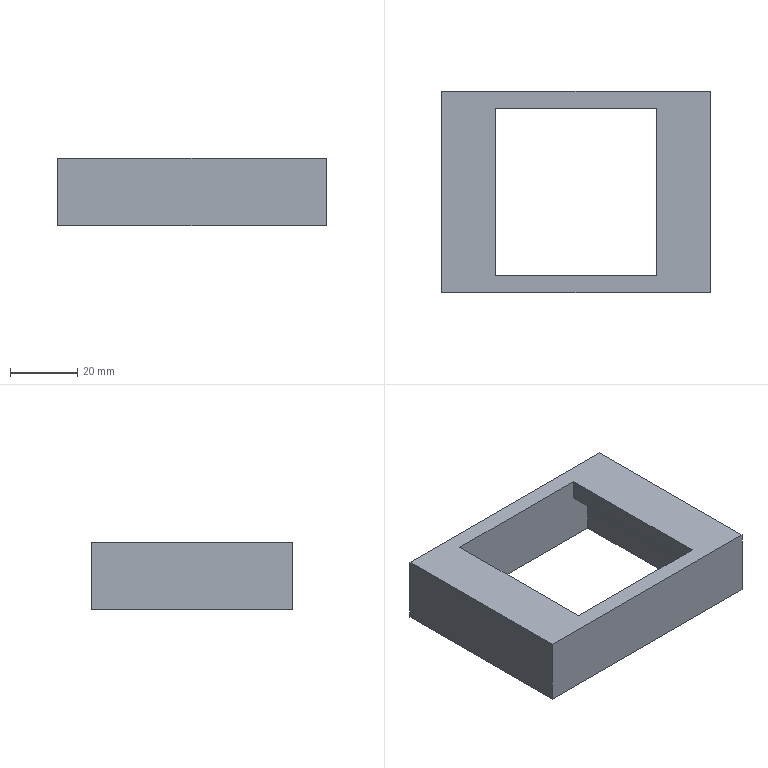Part | SolidWorks | features ICE 2, Extrusion 1 | 1 solid | 14 faces | box 80 x 60 x 20 mm | volume 39600 mm3 | plane 14
STEP:
#1=CARTESIAN_POINT('',(-24.,25.,14.));
#2=VERTEX_POINT('',#1);
#3=CARTESIAN_POINT('',(-24.,-25.,14.));
#4=VERTEX_POINT('',#3);
#5=CARTESIAN_POINT('',(-24.,-25.,14.));
#6=DIRECTION('',(0.,-1.,0.));
#7=VECTOR('',#6,1000.);
#8=LINE('',#5,#7);
#9=EDGE_CURVE('',#2,#4,#8,.T.);
#10=ORIENTED_EDGE('',*,*,#9,.F.);
#11=CARTESIAN_POINT('',(-24.,25.,20.));
#12=VERTEX_POINT('',#11);
#13=CARTESIAN_POINT('',(-24.,25.,-0.001));
#14=DIRECTION('',(0.,0.,1.));
#15=VECTOR('',#14,1000.);
#16=LINE('',#13,#15);
#17=EDGE_CURVE('',#2,#12,#16,.T.);
#18=ORIENTED_EDGE('',*,*,#17,.T.);
#19=CARTESIAN_POINT('',(-24.,-25.,20.));
#20=VERTEX_POINT('',#19);
#21=CARTESIAN_POINT('',(-24.,-25.,20.));
#22=DIRECTION('',(0.,-1.,0.));
#23=VECTOR('',#22,1000.);
#24=LINE('',#21,#23);
#25=EDGE_CURVE('',#12,#20,#24,.T.);
#26=ORIENTED_EDGE('',*,*,#25,.T.);
#27=CARTESIAN_POINT('',(-24.,-25.,-0.001));
#28=DIRECTION('',(0.,0.,1.));
#29=VECTOR('',#28,1000.);
#30=LINE('',#27,#29);
#31=EDGE_CURVE('',#4,#20,#30,.T.);
#32=ORIENTED_EDGE('',*,*,#31,.F.);
#33=EDGE_LOOP('',(#10,#18,#26,#32));
#34=FACE_OUTER_BOUND('',#33,.T.);
#35=CARTESIAN_POINT('',(-24.,-25.,-0.001));
#36=DIRECTION('',(-1.,0.,0.));
#37=DIRECTION('',(0.,0.,1.));
#38=AXIS2_PLACEMENT_3D('',#35,#36,#37);
#39=PLANE('',#38);
#40=ADVANCED_FACE('',(#34),#39,.F.);
#41=CARTESIAN_POINT('',(24.,-25.,14.));
#42=VERTEX_POINT('',#41);
#43=CARTESIAN_POINT('',(24.,25.,14.));
#44=VERTEX_POINT('',#43);
#45=CARTESIAN_POINT('',(24.,-25.,14.));
#46=DIRECTION('',(0.,1.,0.));
#47=VECTOR('',#46,1000.);
#48=LINE('',#45,#47);
#49=EDGE_CURVE('',#42,#44,#48,.T.);
#50=ORIENTED_EDGE('',*,*,#49,.F.);
#51=CARTESIAN_POINT('',(24.,-25.,20.));
#52=VERTEX_POINT('',#51);
#53=CARTESIAN_POINT('',(24.,-25.,-0.001));
#54=DIRECTION('',(0.,0.,1.));
#55=VECTOR('',#54,1000.);
#56=LINE('',#53,#55);
#57=EDGE_CURVE('',#42,#52,#56,.T.);
#58=ORIENTED_EDGE('',*,*,#57,.T.);
#59=CARTESIAN_POINT('',(24.,25.,20.));
#60=VERTEX_POINT('',#59);
#61=CARTESIAN_POINT('',(24.,-25.,20.));
#62=DIRECTION('',(0.,1.,0.));
#63=VECTOR('',#62,1000.);
#64=LINE('',#61,#63);
#65=EDGE_CURVE('',#52,#60,#64,.T.);
#66=ORIENTED_EDGE('',*,*,#65,.T.);
#67=CARTESIAN_POINT('',(24.,25.,-0.001));
#68=DIRECTION('',(0.,0.,1.));
#69=VECTOR('',#68,1000.);
#70=LINE('',#67,#69);
#71=EDGE_CURVE('',#44,#60,#70,.T.);
#72=ORIENTED_EDGE('',*,*,#71,.F.);
#73=EDGE_LOOP('',(#50,#58,#66,#72));
#74=FACE_OUTER_BOUND('',#73,.T.);
#75=CARTESIAN_POINT('',(24.,-25.,-0.001));
#76=DIRECTION('',(1.,0.,0.));
#77=DIRECTION('',(0.,0.,-1.));
#78=AXIS2_PLACEMENT_3D('',#75,#76,#77);
#79=PLANE('',#78);
#80=ADVANCED_FACE('',(#74),#79,.F.);
#81=CARTESIAN_POINT('',(-40.,30.,0.));
#82=VERTEX_POINT('',#81);
#83=CARTESIAN_POINT('',(-40.,-30.,0.));
#84=VERTEX_POINT('',#83);
#85=CARTESIAN_POINT('',(-40.,-30.,0.));
#86=DIRECTION('',(0.,-1.,0.));
#87=VECTOR('',#86,1000.);
#88=LINE('',#85,#87);
#89=EDGE_CURVE('',#82,#84,#88,.T.);
#90=ORIENTED_EDGE('',*,*,#89,.T.);
#91=CARTESIAN_POINT('',(-40.,-30.,20.));
#92=VERTEX_POINT('',#91);
#93=CARTESIAN_POINT('',(-40.,-30.,20.));
#94=DIRECTION('',(0.,0.,-1.));
#95=VECTOR('',#94,1000.);
#96=LINE('',#93,#95);
#97=EDGE_CURVE('',#92,#84,#96,.T.);
#98=ORIENTED_EDGE('',*,*,#97,.F.);
#99=CARTESIAN_POINT('',(-40.,30.,20.));
#100=VERTEX_POINT('',#99);
#101=CARTESIAN_POINT('',(-40.,-30.,20.));
#102=DIRECTION('',(0.,-1.,0.));
#103=VECTOR('',#102,1000.);
#104=LINE('',#101,#103);
#105=EDGE_CURVE('',#100,#92,#104,.T.);
#106=ORIENTED_EDGE('',*,*,#105,.F.);
#107=CARTESIAN_POINT('',(-40.,30.,20.));
#108=DIRECTION('',(0.,0.,-1.));
#109=VECTOR('',#108,1000.);
#110=LINE('',#107,#109);
#111=EDGE_CURVE('',#100,#82,#110,.T.);
#112=ORIENTED_EDGE('',*,*,#111,.T.);
#113=EDGE_LOOP('',(#90,#98,#106,#112));
#114=FACE_OUTER_BOUND('',#113,.T.);
#115=CARTESIAN_POINT('',(-40.,-30.,20.));
#116=DIRECTION('',(1.,0.,0.));
#117=DIRECTION('',(0.,0.,-1.));
#118=AXIS2_PLACEMENT_3D('',#115,#116,#117);
#119=PLANE('',#118);
#120=ADVANCED_FACE('',(#114),#119,.F.);
#121=CARTESIAN_POINT('',(40.,-30.,0.));
#122=VERTEX_POINT('',#121);
#123=CARTESIAN_POINT('',(40.,-30.,0.));
#124=DIRECTION('',(1.,0.,0.));
#125=VECTOR('',#124,1000.);
#126=LINE('',#123,#125);
#127=EDGE_CURVE('',#84,#122,#126,.T.);
#128=ORIENTED_EDGE('',*,*,#127,.T.);
#129=CARTESIAN_POINT('',(40.,-30.,20.));
#130=VERTEX_POINT('',#129);
#131=CARTESIAN_POINT('',(40.,-30.,20.));
#132=DIRECTION('',(0.,0.,-1.));
#133=VECTOR('',#132,1000.);
#134=LINE('',#131,#133);
#135=EDGE_CURVE('',#130,#122,#134,.T.);
#136=ORIENTED_EDGE('',*,*,#135,.F.);
#137=CARTESIAN_POINT('',(40.,-30.,20.));
#138=DIRECTION('',(1.,0.,0.));
#139=VECTOR('',#138,1000.);
#140=LINE('',#137,#139);
#141=EDGE_CURVE('',#92,#130,#140,.T.);
#142=ORIENTED_EDGE('',*,*,#141,.F.);
#143=ORIENTED_EDGE('',*,*,#97,.T.);
#144=EDGE_LOOP('',(#128,#136,#142,#143));
#145=FACE_OUTER_BOUND('',#144,.T.);
#146=CARTESIAN_POINT('',(40.,-30.,20.));
#147=DIRECTION('',(0.,1.,0.));
#148=DIRECTION('',(-1.,0.,0.));
#149=AXIS2_PLACEMENT_3D('',#146,#147,#148);
#150=PLANE('',#149);
#151=ADVANCED_FACE('',(#145),#150,.F.);
#152=CARTESIAN_POINT('',(40.,30.,0.));
#153=VERTEX_POINT('',#152);
#154=CARTESIAN_POINT('',(40.,-30.,0.));
#155=DIRECTION('',(0.,1.,0.));
#156=VECTOR('',#155,1000.);
#157=LINE('',#154,#156);
#158=EDGE_CURVE('',#122,#153,#157,.T.);
#159=ORIENTED_EDGE('',*,*,#158,.T.);
#160=CARTESIAN_POINT('',(40.,30.,20.));
#161=VERTEX_POINT('',#160);
#162=CARTESIAN_POINT('',(40.,30.,20.));
#163=DIRECTION('',(0.,0.,-1.));
#164=VECTOR('',#163,1000.);
#165=LINE('',#162,#164);
#166=EDGE_CURVE('',#161,#153,#165,.T.);
#167=ORIENTED_EDGE('',*,*,#166,.F.);
#168=CARTESIAN_POINT('',(40.,-30.,20.));
#169=DIRECTION('',(0.,1.,0.));
#170=VECTOR('',#169,1000.);
#171=LINE('',#168,#170);
#172=EDGE_CURVE('',#130,#161,#171,.T.);
#173=ORIENTED_EDGE('',*,*,#172,.F.);
#174=ORIENTED_EDGE('',*,*,#135,.T.);
#175=EDGE_LOOP('',(#159,#167,#173,#174));
#176=FACE_OUTER_BOUND('',#175,.T.);
#177=CARTESIAN_POINT('',(40.,-30.,20.));
#178=DIRECTION('',(-1.,0.,0.));
#179=DIRECTION('',(0.,0.,1.));
#180=AXIS2_PLACEMENT_3D('',#177,#178,#179);
#181=PLANE('',#180);
#182=ADVANCED_FACE('',(#176),#181,.F.);
#183=CARTESIAN_POINT('',(40.,30.,0.));
#184=DIRECTION('',(-1.,0.,0.));
#185=VECTOR('',#184,1000.);
#186=LINE('',#183,#185);
#187=EDGE_CURVE('',#153,#82,#186,.T.);
#188=ORIENTED_EDGE('',*,*,#187,.T.);
#189=ORIENTED_EDGE('',*,*,#111,.F.);
#190=CARTESIAN_POINT('',(40.,30.,20.));
#191=DIRECTION('',(-1.,0.,0.));
#192=VECTOR('',#191,1000.);
#193=LINE('',#190,#192);
#194=EDGE_CURVE('',#161,#100,#193,.T.);
#195=ORIENTED_EDGE('',*,*,#194,.F.);
#196=ORIENTED_EDGE('',*,*,#166,.T.);
#197=EDGE_LOOP('',(#188,#189,#195,#196));
#198=FACE_OUTER_BOUND('',#197,.T.);
#199=CARTESIAN_POINT('',(40.,30.,20.));
#200=DIRECTION('',(0.,-1.,0.));
#201=DIRECTION('',(1.,0.,0.));
#202=AXIS2_PLACEMENT_3D('',#199,#200,#201);
#203=PLANE('',#202);
#204=ADVANCED_FACE('',(#198),#203,.F.);
#205=ORIENTED_EDGE('',*,*,#25,.F.);
#206=CARTESIAN_POINT('',(24.,25.,20.));
#207=DIRECTION('',(-1.,0.,0.));
#208=VECTOR('',#207,1000.);
#209=LINE('',#206,#208);
#210=EDGE_CURVE('',#60,#12,#209,.T.);
#211=ORIENTED_EDGE('',*,*,#210,.F.);
#212=ORIENTED_EDGE('',*,*,#65,.F.);
#213=CARTESIAN_POINT('',(24.,-25.,20.));
#214=DIRECTION('',(1.,0.,0.));
#215=VECTOR('',#214,1000.);
#216=LINE('',#213,#215);
#217=EDGE_CURVE('',#20,#52,#216,.T.);
#218=ORIENTED_EDGE('',*,*,#217,.F.);
#219=EDGE_LOOP('',(#205,#211,#212,#218));
#220=FACE_BOUND('',#219,.T.);
#221=ORIENTED_EDGE('',*,*,#105,.T.);
#222=ORIENTED_EDGE('',*,*,#141,.T.);
#223=ORIENTED_EDGE('',*,*,#172,.T.);
#224=ORIENTED_EDGE('',*,*,#194,.T.);
#225=EDGE_LOOP('',(#221,#222,#223,#224));
#226=FACE_OUTER_BOUND('',#225,.T.);
#227=CARTESIAN_POINT('',(0.,0.,20.));
#228=DIRECTION('',(0.,0.,1.));
#229=DIRECTION('',(1.,0.,0.));
#230=AXIS2_PLACEMENT_3D('',#227,#228,#229);
#231=PLANE('',#230);
#232=ADVANCED_FACE('',(#220,#226),#231,.T.);
#233=CARTESIAN_POINT('',(-30.,25.,0.));
#234=VERTEX_POINT('',#233);
#235=CARTESIAN_POINT('',(30.,25.,0.));
#236=VERTEX_POINT('',#235);
#237=CARTESIAN_POINT('',(24.,25.,0.));
#238=DIRECTION('',(1.,0.,0.));
#239=VECTOR('',#238,1000.);
#240=LINE('',#237,#239);
#241=EDGE_CURVE('',#234,#236,#240,.T.);
#242=ORIENTED_EDGE('',*,*,#241,.F.);
#243=CARTESIAN_POINT('',(-30.,-25.,0.));
#244=VERTEX_POINT('',#243);
#245=CARTESIAN_POINT('',(-30.,-25.,0.));
#246=DIRECTION('',(0.,1.,0.));
#247=VECTOR('',#246,1000.);
#248=LINE('',#245,#247);
#249=EDGE_CURVE('',#244,#234,#248,.T.);
#250=ORIENTED_EDGE('',*,*,#249,.F.);
#251=CARTESIAN_POINT('',(30.,-25.,0.));
#252=VERTEX_POINT('',#251);
#253=CARTESIAN_POINT('',(24.,-25.,0.));
#254=DIRECTION('',(-1.,0.,0.));
#255=VECTOR('',#254,1000.);
#256=LINE('',#253,#255);
#257=EDGE_CURVE('',#252,#244,#256,.T.);
#258=ORIENTED_EDGE('',*,*,#257,.F.);
#259=CARTESIAN_POINT('',(30.,-25.,0.));
#260=DIRECTION('',(0.,-1.,0.));
#261=VECTOR('',#260,1000.);
#262=LINE('',#259,#261);
#263=EDGE_CURVE('',#236,#252,#262,.T.);
#264=ORIENTED_EDGE('',*,*,#263,.F.);
#265=EDGE_LOOP('',(#242,#250,#258,#264));
#266=FACE_BOUND('',#265,.T.);
#267=ORIENTED_EDGE('',*,*,#89,.F.);
#268=ORIENTED_EDGE('',*,*,#187,.F.);
#269=ORIENTED_EDGE('',*,*,#158,.F.);
#270=ORIENTED_EDGE('',*,*,#127,.F.);
#271=EDGE_LOOP('',(#267,#268,#269,#270));
#272=FACE_OUTER_BOUND('',#271,.T.);
#273=CARTESIAN_POINT('',(0.,0.,0.));
#274=DIRECTION('',(0.,0.,1.));
#275=DIRECTION('',(1.,0.,0.));
#276=AXIS2_PLACEMENT_3D('',#273,#274,#275);
#277=PLANE('',#276);
#278=ADVANCED_FACE('',(#266,#272),#277,.F.);
#279=ORIENTED_EDGE('',*,*,#241,.T.);
#280=CARTESIAN_POINT('',(30.,25.,14.));
#281=VERTEX_POINT('',#280);
#282=CARTESIAN_POINT('',(30.,25.,14.));
#283=DIRECTION('',(0.,0.,-1.));
#284=VECTOR('',#283,1000.);
#285=LINE('',#282,#284);
#286=EDGE_CURVE('',#281,#236,#285,.T.);
#287=ORIENTED_EDGE('',*,*,#286,.F.);
#288=CARTESIAN_POINT('',(-30.,25.,14.));
#289=DIRECTION('',(1.,0.,0.));
#290=VECTOR('',#289,1000.);
#291=LINE('',#288,#290);
#292=EDGE_CURVE('',#44,#281,#291,.T.);
#293=ORIENTED_EDGE('',*,*,#292,.F.);
#294=ORIENTED_EDGE('',*,*,#71,.T.);
#295=ORIENTED_EDGE('',*,*,#210,.T.);
#296=ORIENTED_EDGE('',*,*,#17,.F.);
#297=CARTESIAN_POINT('',(-30.,25.,14.));
#298=VERTEX_POINT('',#297);
#299=CARTESIAN_POINT('',(-30.,25.,14.));
#300=DIRECTION('',(1.,0.,0.));
#301=VECTOR('',#300,1000.);
#302=LINE('',#299,#301);
#303=EDGE_CURVE('',#298,#2,#302,.T.);
#304=ORIENTED_EDGE('',*,*,#303,.F.);
#305=CARTESIAN_POINT('',(-30.,25.,14.));
#306=DIRECTION('',(0.,0.,-1.));
#307=VECTOR('',#306,1000.);
#308=LINE('',#305,#307);
#309=EDGE_CURVE('',#298,#234,#308,.T.);
#310=ORIENTED_EDGE('',*,*,#309,.T.);
#311=EDGE_LOOP('',(#279,#287,#293,#294,#295,#296,#304,#310));
#312=FACE_OUTER_BOUND('',#311,.T.);
#313=CARTESIAN_POINT('',(24.,25.,-0.001));
#314=DIRECTION('',(0.,1.,0.));
#315=DIRECTION('',(-1.,0.,0.));
#316=AXIS2_PLACEMENT_3D('',#313,#314,#315);
#317=PLANE('',#316);
#318=ADVANCED_FACE('',(#312),#317,.F.);
#319=ORIENTED_EDGE('',*,*,#257,.T.);
#320=CARTESIAN_POINT('',(-30.,-25.,14.));
#321=VERTEX_POINT('',#320);
#322=CARTESIAN_POINT('',(-30.,-25.,14.));
#323=DIRECTION('',(0.,0.,-1.));
#324=VECTOR('',#323,1000.);
#325=LINE('',#322,#324);
#326=EDGE_CURVE('',#321,#244,#325,.T.);
#327=ORIENTED_EDGE('',*,*,#326,.F.);
#328=CARTESIAN_POINT('',(-30.,-25.,14.));
#329=DIRECTION('',(-1.,0.,0.));
#330=VECTOR('',#329,1000.);
#331=LINE('',#328,#330);
#332=EDGE_CURVE('',#4,#321,#331,.T.);
#333=ORIENTED_EDGE('',*,*,#332,.F.);
#334=ORIENTED_EDGE('',*,*,#31,.T.);
#335=ORIENTED_EDGE('',*,*,#217,.T.);
#336=ORIENTED_EDGE('',*,*,#57,.F.);
#337=CARTESIAN_POINT('',(30.,-25.,14.));
#338=VERTEX_POINT('',#337);
#339=CARTESIAN_POINT('',(-30.,-25.,14.));
#340=DIRECTION('',(-1.,0.,0.));
#341=VECTOR('',#340,1000.);
#342=LINE('',#339,#341);
#343=EDGE_CURVE('',#338,#42,#342,.T.);
#344=ORIENTED_EDGE('',*,*,#343,.F.);
#345=CARTESIAN_POINT('',(30.,-25.,14.));
#346=DIRECTION('',(0.,0.,-1.));
#347=VECTOR('',#346,1000.);
#348=LINE('',#345,#347);
#349=EDGE_CURVE('',#338,#252,#348,.T.);
#350=ORIENTED_EDGE('',*,*,#349,.T.);
#351=EDGE_LOOP('',(#319,#327,#333,#334,#335,#336,#344,#350));
#352=FACE_OUTER_BOUND('',#351,.T.);
#353=CARTESIAN_POINT('',(24.,-25.,-0.001));
#354=DIRECTION('',(0.,-1.,0.));
#355=DIRECTION('',(1.,0.,0.));
#356=AXIS2_PLACEMENT_3D('',#353,#354,#355);
#357=PLANE('',#356);
#358=ADVANCED_FACE('',(#352),#357,.F.);
#359=ORIENTED_EDGE('',*,*,#49,.T.);
#360=ORIENTED_EDGE('',*,*,#292,.T.);
#361=CARTESIAN_POINT('',(30.,-25.,14.));
#362=DIRECTION('',(0.,-1.,0.));
#363=VECTOR('',#362,1000.);
#364=LINE('',#361,#363);
#365=EDGE_CURVE('',#281,#338,#364,.T.);
#366=ORIENTED_EDGE('',*,*,#365,.T.);
#367=ORIENTED_EDGE('',*,*,#343,.T.);
#368=EDGE_LOOP('',(#359,#360,#366,#367));
#369=FACE_OUTER_BOUND('',#368,.T.);
#370=CARTESIAN_POINT('',(0.,0.,14.));
#371=DIRECTION('',(0.,0.,-1.));
#372=DIRECTION('',(-1.,0.,0.));
#373=AXIS2_PLACEMENT_3D('',#370,#371,#372);
#374=PLANE('',#373);
#375=ADVANCED_FACE('',(#369),#374,.T.);
#376=ORIENTED_EDGE('',*,*,#263,.T.);
#377=ORIENTED_EDGE('',*,*,#349,.F.);
#378=ORIENTED_EDGE('',*,*,#365,.F.);
#379=ORIENTED_EDGE('',*,*,#286,.T.);
#380=EDGE_LOOP('',(#376,#377,#378,#379));
#381=FACE_OUTER_BOUND('',#380,.T.);
#382=CARTESIAN_POINT('',(30.,-25.,14.));
#383=DIRECTION('',(1.,0.,0.));
#384=DIRECTION('',(0.,0.,-1.));
#385=AXIS2_PLACEMENT_3D('',#382,#383,#384);
#386=PLANE('',#385);
#387=ADVANCED_FACE('',(#381),#386,.F.);
#388=ORIENTED_EDGE('',*,*,#9,.T.);
#389=ORIENTED_EDGE('',*,*,#332,.T.);
#390=CARTESIAN_POINT('',(-30.,-25.,14.));
#391=DIRECTION('',(0.,1.,0.));
#392=VECTOR('',#391,1000.);
#393=LINE('',#390,#392);
#394=EDGE_CURVE('',#321,#298,#393,.T.);
#395=ORIENTED_EDGE('',*,*,#394,.T.);
#396=ORIENTED_EDGE('',*,*,#303,.T.);
#397=EDGE_LOOP('',(#388,#389,#395,#396));
#398=FACE_OUTER_BOUND('',#397,.T.);
#399=CARTESIAN_POINT('',(0.,0.,14.));
#400=DIRECTION('',(0.,0.,-1.));
#401=DIRECTION('',(-1.,0.,0.));
#402=AXIS2_PLACEMENT_3D('',#399,#400,#401);
#403=PLANE('',#402);
#404=ADVANCED_FACE('',(#398),#403,.T.);
#405=ORIENTED_EDGE('',*,*,#249,.T.);
#406=ORIENTED_EDGE('',*,*,#309,.F.);
#407=ORIENTED_EDGE('',*,*,#394,.F.);
#408=ORIENTED_EDGE('',*,*,#326,.T.);
#409=EDGE_LOOP('',(#405,#406,#407,#408));
#410=FACE_OUTER_BOUND('',#409,.T.);
#411=CARTESIAN_POINT('',(-30.,-25.,14.));
#412=DIRECTION('',(-1.,0.,0.));
#413=DIRECTION('',(0.,0.,1.));
#414=AXIS2_PLACEMENT_3D('',#411,#412,#413);
#415=PLANE('',#414);
#416=ADVANCED_FACE('',(#410),#415,.F.);
#417=CLOSED_SHELL('',(#40,#80,#120,#151,#182,#204,#232,#278,#318,#358,#375,#387,#404,#416));
#418=MANIFOLD_SOLID_BREP('',#417);
#419=CARTESIAN_POINT('',(0.,0.,0.));
#420=DIRECTION('',(0.,0.,1.));
#421=DIRECTION('',(1.,0.,0.));
#422=AXIS2_PLACEMENT_3D('',#419,#420,#421);
#423=(LENGTH_UNIT()NAMED_UNIT(*)SI_UNIT(.MILLI.,.METRE.));
#424=UNCERTAINTY_MEASURE_WITH_UNIT(LENGTH_MEASURE(0.00001),#423,'','');
#425=(NAMED_UNIT(*)PLANE_ANGLE_UNIT()SI_UNIT($,.RADIAN.));
#426=(NAMED_UNIT(*)SI_UNIT($,.STERADIAN.)SOLID_ANGLE_UNIT());
#427=(GEOMETRIC_REPRESENTATION_CONTEXT(3)GLOBAL_UNCERTAINTY_ASSIGNED_CONTEXT((#424))GLOBAL_UNIT_ASSIGNED_CONTEXT((#423,#425,#426))REPRESENTATION_CONTEXT('',''));
#428=ADVANCED_BREP_SHAPE_REPRESENTATION('',(#418,#422),#427);